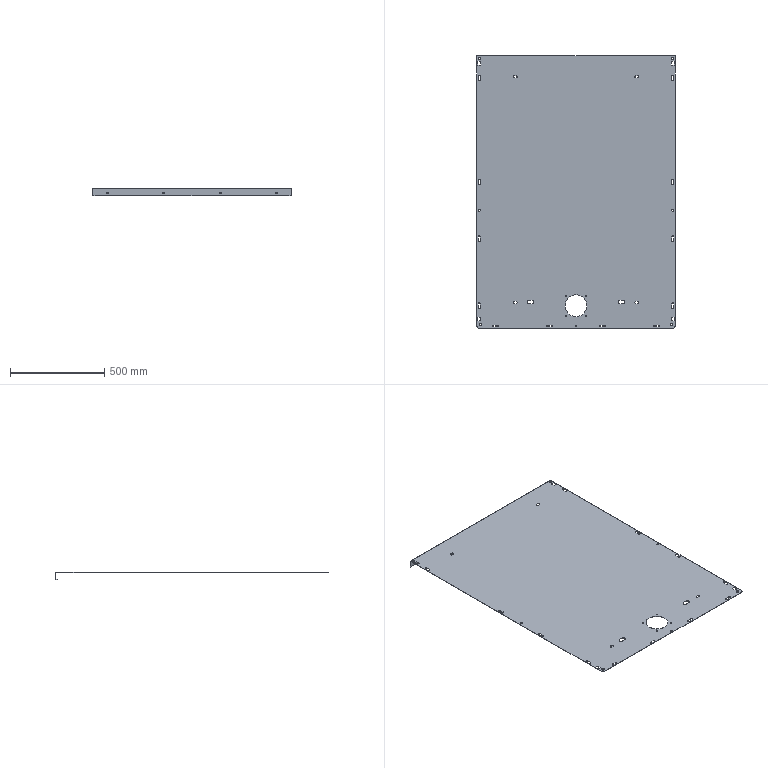Part | SolidWorks | features Cut 5, ICE 4, EdgeFlange 2, Fillet 1, FlatPattern 1, SMBaseFlange 1, SheetMetal 1 | 1 solid | 162 faces | box 1050 x 1445 x 39.5 mm | volume 2316443 mm3 | cylinder 84 | plane 78 | commonest cylinder face diameters 10 x34 11 x16 5.9 x8 10.5 x8 20 x6 12.8 x4